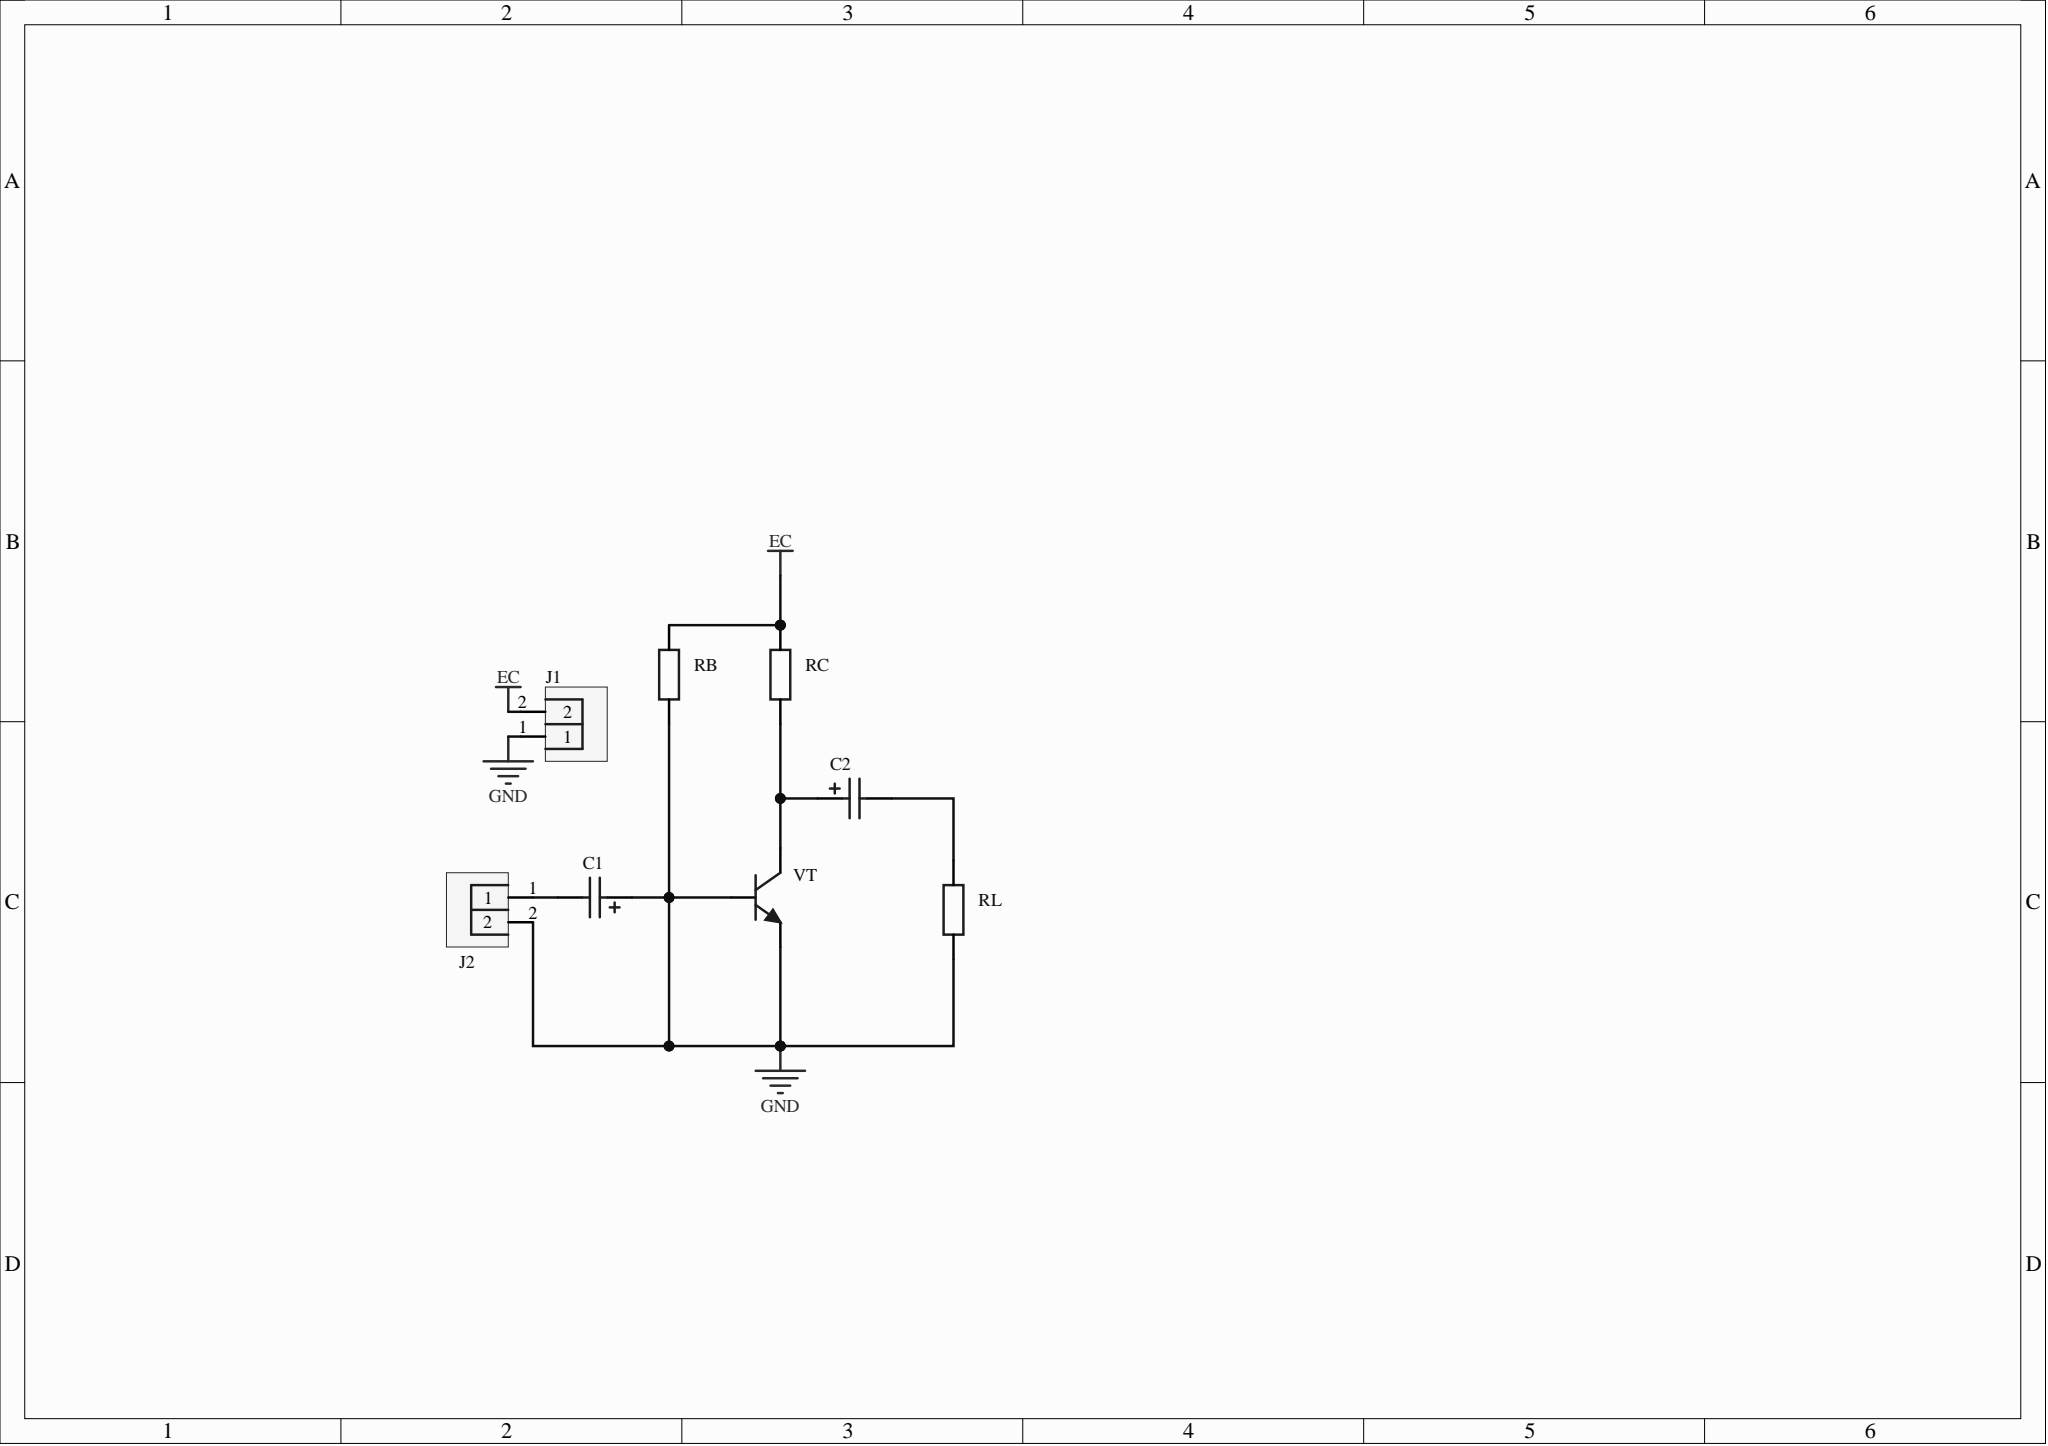Circuit board | Altium Designer | 8 parts | 5 nets
Bill of materials:
Comment,Description,Designator,Footprint,LibRef,Quantity
"100pF","","C1, C2","C_Ele_SMD_3x5.4mm","C_Ele_SMD_3x5.4mm","2"
"","","J1, J2","HDR-TH_2P-P2.54-V-M-1","HDR-M_2.54_1x2P","2"
"5.1K","","RB","R0603","Res_0603","1"
"1K","","RC, RL","R0603","Res_0603","2"
"","","VT","S8050_SOT-23","S8050_SOT_NPN","1"
Netlist (Protel format):
[
C1
C_Ele_SMD_3x5.4mm
100pF



]
[
C2
C_Ele_SMD_3x5.4mm
100pF



]
[
J1
HDR-TH_2P-P2.54-V-M-1




]
[
J2
HDR-TH_2P-P2.54-V-M-1




]
[
RB
R0603
5.1K



]
[
RC
R0603
1K



]
[
RL
R0603
1K



]
[
VT
S8050_SOT-23




]
(
NetC2_2
C2-2
RL-2
)
(
NetC2_1
C2-1
RC-1
VT-3
)
(
NetC1_2
C1-2
J2-1
)
(
GND
C1-1
J1-1
J2-2
RB-1
RL-1
VT-1
VT-2
)
(
EC
J1-2
RB-2
RC-2
)